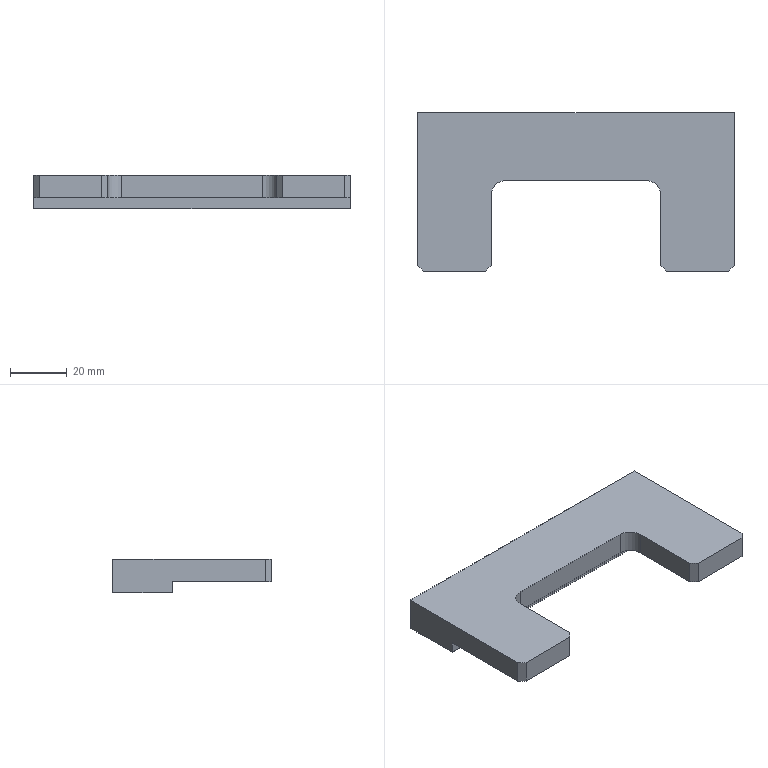Part | SolidWorks | features ICE 2, Chamfer 1, Extrusion 1, Fillet 1, HoleWzd 1 | 1 solid | 30 faces | box 112 x 56 x 12 mm | volume 43333 mm3 | plane 16 | cylinder 8 | cone 6 | commonest cylinder face diameters 5 x6 10 x2
STEP:
#1=CARTESIAN_POINT('',(6.,41.,3.5));
#2=VERTEX_POINT('',#1);
#3=CARTESIAN_POINT('',(6.,41.,8.5));
#4=VERTEX_POINT('',#3);
#5=CARTESIAN_POINT('',(6.,41.,6.));
#6=DIRECTION('',(0.,1.,0.));
#7=DIRECTION('',(0.,0.,1.));
#8=AXIS2_PLACEMENT_3D('',#5,#6,#7);
#9=CIRCLE('',#8,2.5);
#10=EDGE_CURVE('',#2,#4,#9,.T.);
#11=ORIENTED_EDGE('',*,*,#10,.F.);
#12=CARTESIAN_POINT('',(6.,56.,3.5));
#13=VERTEX_POINT('',#12);
#14=CARTESIAN_POINT('',(6.,56.,3.5));
#15=DIRECTION('',(0.,1.,0.));
#16=VECTOR('',#15,1000.);
#17=LINE('',#14,#16);
#18=EDGE_CURVE('',#2,#13,#17,.T.);
#19=ORIENTED_EDGE('',*,*,#18,.T.);
#20=CARTESIAN_POINT('',(6.,56.,8.5));
#21=VERTEX_POINT('',#20);
#22=CARTESIAN_POINT('',(6.,56.,6.));
#23=DIRECTION('',(0.,1.,0.));
#24=DIRECTION('',(0.,0.,1.));
#25=AXIS2_PLACEMENT_3D('',#22,#23,#24);
#26=CIRCLE('',#25,2.5);
#27=EDGE_CURVE('',#13,#21,#26,.T.);
#28=ORIENTED_EDGE('',*,*,#27,.T.);
#29=CARTESIAN_POINT('',(6.,56.,8.5));
#30=DIRECTION('',(0.,1.,0.));
#31=VECTOR('',#30,1000.);
#32=LINE('',#29,#31);
#33=EDGE_CURVE('',#4,#21,#32,.T.);
#34=ORIENTED_EDGE('',*,*,#33,.F.);
#35=EDGE_LOOP('',(#11,#19,#28,#34));
#36=FACE_OUTER_BOUND('',#35,.T.);
#37=CARTESIAN_POINT('',(6.,56.,6.));
#38=DIRECTION('',(0.,1.,0.));
#39=DIRECTION('',(0.,0.,1.));
#40=AXIS2_PLACEMENT_3D('',#37,#38,#39);
#41=CYLINDRICAL_SURFACE('',#40,2.5);
#42=ADVANCED_FACE('',(#36),#41,.F.);
#43=CARTESIAN_POINT('',(6.,39.498,6.));
#44=VERTEX_POINT('',#43);
#45=CARTESIAN_POINT('',(6.,41.,8.5));
#46=DIRECTION('',(0.,0.515,0.8572));
#47=VECTOR('',#46,1000.);
#48=LINE('',#45,#47);
#49=EDGE_CURVE('',#44,#4,#48,.T.);
#50=ORIENTED_EDGE('',*,*,#49,.F.);
#51=CARTESIAN_POINT('',(6.,41.,3.5));
#52=DIRECTION('',(0.,0.515,-0.8572));
#53=VECTOR('',#52,1000.);
#54=LINE('',#51,#53);
#55=EDGE_CURVE('',#44,#2,#54,.T.);
#56=ORIENTED_EDGE('',*,*,#55,.T.);
#57=ORIENTED_EDGE('',*,*,#10,.T.);
#58=EDGE_LOOP('',(#50,#56,#57));
#59=FACE_OUTER_BOUND('',#58,.T.);
#60=CARTESIAN_POINT('',(6.,41.,6.));
#61=DIRECTION('',(0.,1.,0.));
#62=DIRECTION('',(0.,0.,1.));
#63=AXIS2_PLACEMENT_3D('',#60,#61,#62);
#64=CONICAL_SURFACE('',#63,2.5,1.03);
#65=ADVANCED_FACE('',(#59),#64,.F.);
#66=CARTESIAN_POINT('',(56.,41.,3.5));
#67=VERTEX_POINT('',#66);
#68=CARTESIAN_POINT('',(56.,41.,8.5));
#69=VERTEX_POINT('',#68);
#70=CARTESIAN_POINT('',(56.,41.,6.));
#71=DIRECTION('',(0.,1.,0.));
#72=DIRECTION('',(0.,0.,1.));
#73=AXIS2_PLACEMENT_3D('',#70,#71,#72);
#74=CIRCLE('',#73,2.5);
#75=EDGE_CURVE('',#67,#69,#74,.T.);
#76=ORIENTED_EDGE('',*,*,#75,.F.);
#77=CARTESIAN_POINT('',(56.,56.,3.5));
#78=VERTEX_POINT('',#77);
#79=CARTESIAN_POINT('',(56.,56.,3.5));
#80=DIRECTION('',(0.,1.,0.));
#81=VECTOR('',#80,1000.);
#82=LINE('',#79,#81);
#83=EDGE_CURVE('',#67,#78,#82,.T.);
#84=ORIENTED_EDGE('',*,*,#83,.T.);
#85=CARTESIAN_POINT('',(56.,56.,8.5));
#86=VERTEX_POINT('',#85);
#87=CARTESIAN_POINT('',(56.,56.,6.));
#88=DIRECTION('',(0.,1.,0.));
#89=DIRECTION('',(0.,0.,1.));
#90=AXIS2_PLACEMENT_3D('',#87,#88,#89);
#91=CIRCLE('',#90,2.5);
#92=EDGE_CURVE('',#78,#86,#91,.T.);
#93=ORIENTED_EDGE('',*,*,#92,.T.);
#94=CARTESIAN_POINT('',(56.,56.,8.5));
#95=DIRECTION('',(0.,1.,0.));
#96=VECTOR('',#95,1000.);
#97=LINE('',#94,#96);
#98=EDGE_CURVE('',#69,#86,#97,.T.);
#99=ORIENTED_EDGE('',*,*,#98,.F.);
#100=EDGE_LOOP('',(#76,#84,#93,#99));
#101=FACE_OUTER_BOUND('',#100,.T.);
#102=CARTESIAN_POINT('',(56.,56.,6.));
#103=DIRECTION('',(0.,1.,0.));
#104=DIRECTION('',(0.,0.,1.));
#105=AXIS2_PLACEMENT_3D('',#102,#103,#104);
#106=CYLINDRICAL_SURFACE('',#105,2.5);
#107=ADVANCED_FACE('',(#101),#106,.F.);
#108=CARTESIAN_POINT('',(56.,39.498,6.));
#109=VERTEX_POINT('',#108);
#110=CARTESIAN_POINT('',(56.,41.,8.5));
#111=DIRECTION('',(0.,0.515,0.8572));
#112=VECTOR('',#111,1000.);
#113=LINE('',#110,#112);
#114=EDGE_CURVE('',#109,#69,#113,.T.);
#115=ORIENTED_EDGE('',*,*,#114,.F.);
#116=CARTESIAN_POINT('',(56.,41.,3.5));
#117=DIRECTION('',(0.,0.515,-0.8572));
#118=VECTOR('',#117,1000.);
#119=LINE('',#116,#118);
#120=EDGE_CURVE('',#109,#67,#119,.T.);
#121=ORIENTED_EDGE('',*,*,#120,.T.);
#122=ORIENTED_EDGE('',*,*,#75,.T.);
#123=EDGE_LOOP('',(#115,#121,#122));
#124=FACE_OUTER_BOUND('',#123,.T.);
#125=CARTESIAN_POINT('',(56.,41.,6.));
#126=DIRECTION('',(0.,1.,0.));
#127=DIRECTION('',(0.,0.,1.));
#128=AXIS2_PLACEMENT_3D('',#125,#126,#127);
#129=CONICAL_SURFACE('',#128,2.5,1.03);
#130=ADVANCED_FACE('',(#124),#129,.F.);
#131=CARTESIAN_POINT('',(106.,41.,3.5));
#132=VERTEX_POINT('',#131);
#133=CARTESIAN_POINT('',(106.,41.,8.5));
#134=VERTEX_POINT('',#133);
#135=CARTESIAN_POINT('',(106.,41.,6.));
#136=DIRECTION('',(0.,1.,0.));
#137=DIRECTION('',(0.,0.,1.));
#138=AXIS2_PLACEMENT_3D('',#135,#136,#137);
#139=CIRCLE('',#138,2.5);
#140=EDGE_CURVE('',#132,#134,#139,.T.);
#141=ORIENTED_EDGE('',*,*,#140,.F.);
#142=CARTESIAN_POINT('',(106.,56.,3.5));
#143=VERTEX_POINT('',#142);
#144=CARTESIAN_POINT('',(106.,56.,3.5));
#145=DIRECTION('',(0.,1.,0.));
#146=VECTOR('',#145,1000.);
#147=LINE('',#144,#146);
#148=EDGE_CURVE('',#132,#143,#147,.T.);
#149=ORIENTED_EDGE('',*,*,#148,.T.);
#150=CARTESIAN_POINT('',(106.,56.,8.5));
#151=VERTEX_POINT('',#150);
#152=CARTESIAN_POINT('',(106.,56.,6.));
#153=DIRECTION('',(0.,1.,0.));
#154=DIRECTION('',(0.,0.,1.));
#155=AXIS2_PLACEMENT_3D('',#152,#153,#154);
#156=CIRCLE('',#155,2.5);
#157=EDGE_CURVE('',#143,#151,#156,.T.);
#158=ORIENTED_EDGE('',*,*,#157,.T.);
#159=CARTESIAN_POINT('',(106.,56.,8.5));
#160=DIRECTION('',(0.,1.,0.));
#161=VECTOR('',#160,1000.);
#162=LINE('',#159,#161);
#163=EDGE_CURVE('',#134,#151,#162,.T.);
#164=ORIENTED_EDGE('',*,*,#163,.F.);
#165=EDGE_LOOP('',(#141,#149,#158,#164));
#166=FACE_OUTER_BOUND('',#165,.T.);
#167=CARTESIAN_POINT('',(106.,56.,6.));
#168=DIRECTION('',(0.,1.,0.));
#169=DIRECTION('',(0.,0.,1.));
#170=AXIS2_PLACEMENT_3D('',#167,#168,#169);
#171=CYLINDRICAL_SURFACE('',#170,2.5);
#172=ADVANCED_FACE('',(#166),#171,.F.);
#173=CARTESIAN_POINT('',(106.,39.498,6.));
#174=VERTEX_POINT('',#173);
#175=CARTESIAN_POINT('',(106.,41.,8.5));
#176=DIRECTION('',(0.,0.515,0.8572));
#177=VECTOR('',#176,1000.);
#178=LINE('',#175,#177);
#179=EDGE_CURVE('',#174,#134,#178,.T.);
#180=ORIENTED_EDGE('',*,*,#179,.F.);
#181=CARTESIAN_POINT('',(106.,41.,3.5));
#182=DIRECTION('',(0.,0.515,-0.8572));
#183=VECTOR('',#182,1000.);
#184=LINE('',#181,#183);
#185=EDGE_CURVE('',#174,#132,#184,.T.);
#186=ORIENTED_EDGE('',*,*,#185,.T.);
#187=ORIENTED_EDGE('',*,*,#140,.T.);
#188=EDGE_LOOP('',(#180,#186,#187));
#189=FACE_OUTER_BOUND('',#188,.T.);
#190=CARTESIAN_POINT('',(106.,41.,6.));
#191=DIRECTION('',(0.,1.,0.));
#192=DIRECTION('',(0.,0.,1.));
#193=AXIS2_PLACEMENT_3D('',#190,#191,#192);
#194=CONICAL_SURFACE('',#193,2.5,1.03);
#195=ADVANCED_FACE('',(#189),#194,.F.);
#196=CARTESIAN_POINT('',(88.,0.,12.));
#197=VERTEX_POINT('',#196);
#198=CARTESIAN_POINT('',(110.,0.,12.));
#199=VERTEX_POINT('',#198);
#200=CARTESIAN_POINT('',(0.,0.,12.));
#201=DIRECTION('',(1.,0.,0.));
#202=VECTOR('',#201,1000.);
#203=LINE('',#200,#202);
#204=EDGE_CURVE('',#197,#199,#203,.T.);
#205=ORIENTED_EDGE('',*,*,#204,.F.);
#206=CARTESIAN_POINT('',(88.,0.,4.));
#207=VERTEX_POINT('',#206);
#208=CARTESIAN_POINT('',(88.,0.,12.));
#209=DIRECTION('',(0.,0.,-1.));
#210=VECTOR('',#209,1000.);
#211=LINE('',#208,#210);
#212=EDGE_CURVE('',#197,#207,#211,.T.);
#213=ORIENTED_EDGE('',*,*,#212,.T.);
#214=CARTESIAN_POINT('',(110.,0.,4.));
#215=VERTEX_POINT('',#214);
#216=CARTESIAN_POINT('',(112.,0.,4.));
#217=DIRECTION('',(-1.,0.,0.));
#218=VECTOR('',#217,1000.);
#219=LINE('',#216,#218);
#220=EDGE_CURVE('',#215,#207,#219,.T.);
#221=ORIENTED_EDGE('',*,*,#220,.F.);
#222=CARTESIAN_POINT('',(110.,0.,12.));
#223=DIRECTION('',(0.,0.,1.));
#224=VECTOR('',#223,1000.);
#225=LINE('',#222,#224);
#226=EDGE_CURVE('',#215,#199,#225,.T.);
#227=ORIENTED_EDGE('',*,*,#226,.T.);
#228=EDGE_LOOP('',(#205,#213,#221,#227));
#229=FACE_OUTER_BOUND('',#228,.T.);
#230=CARTESIAN_POINT('',(0.,0.,12.));
#231=DIRECTION('',(0.,1.,0.));
#232=DIRECTION('',(0.,0.,1.));
#233=AXIS2_PLACEMENT_3D('',#230,#231,#232);
#234=PLANE('',#233);
#235=ADVANCED_FACE('',(#229),#234,.F.);
#236=CARTESIAN_POINT('',(0.,2.,4.));
#237=VERTEX_POINT('',#236);
#238=CARTESIAN_POINT('',(0.,35.,4.));
#239=VERTEX_POINT('',#238);
#240=CARTESIAN_POINT('',(0.,0.,4.));
#241=DIRECTION('',(0.,1.,0.));
#242=VECTOR('',#241,1000.);
#243=LINE('',#240,#242);
#244=EDGE_CURVE('',#237,#239,#243,.T.);
#245=ORIENTED_EDGE('',*,*,#244,.F.);
#246=CARTESIAN_POINT('',(0.,2.,12.));
#247=VERTEX_POINT('',#246);
#248=CARTESIAN_POINT('',(0.,2.,12.));
#249=DIRECTION('',(0.,0.,1.));
#250=VECTOR('',#249,1000.);
#251=LINE('',#248,#250);
#252=EDGE_CURVE('',#237,#247,#251,.T.);
#253=ORIENTED_EDGE('',*,*,#252,.T.);
#254=CARTESIAN_POINT('',(0.,56.,12.));
#255=VERTEX_POINT('',#254);
#256=CARTESIAN_POINT('',(0.,0.,12.));
#257=DIRECTION('',(0.,-1.,0.));
#258=VECTOR('',#257,1000.);
#259=LINE('',#256,#258);
#260=EDGE_CURVE('',#255,#247,#259,.T.);
#261=ORIENTED_EDGE('',*,*,#260,.F.);
#262=CARTESIAN_POINT('',(0.,56.,0.));
#263=VERTEX_POINT('',#262);
#264=CARTESIAN_POINT('',(0.,56.,12.));
#265=DIRECTION('',(0.,0.,-1.));
#266=VECTOR('',#265,1000.);
#267=LINE('',#264,#266);
#268=EDGE_CURVE('',#255,#263,#267,.T.);
#269=ORIENTED_EDGE('',*,*,#268,.T.);
#270=CARTESIAN_POINT('',(0.,35.,0.));
#271=VERTEX_POINT('',#270);
#272=CARTESIAN_POINT('',(0.,0.,0.));
#273=DIRECTION('',(0.,-1.,0.));
#274=VECTOR('',#273,1000.);
#275=LINE('',#272,#274);
#276=EDGE_CURVE('',#263,#271,#275,.T.);
#277=ORIENTED_EDGE('',*,*,#276,.T.);
#278=CARTESIAN_POINT('',(0.,35.,4.));
#279=DIRECTION('',(0.,0.,-1.));
#280=VECTOR('',#279,1000.);
#281=LINE('',#278,#280);
#282=EDGE_CURVE('',#239,#271,#281,.T.);
#283=ORIENTED_EDGE('',*,*,#282,.F.);
#284=EDGE_LOOP('',(#245,#253,#261,#269,#277,#283));
#285=FACE_OUTER_BOUND('',#284,.T.);
#286=CARTESIAN_POINT('',(0.,0.,12.));
#287=DIRECTION('',(1.,0.,0.));
#288=DIRECTION('',(0.,0.,-1.));
#289=AXIS2_PLACEMENT_3D('',#286,#287,#288);
#290=PLANE('',#289);
#291=ADVANCED_FACE('',(#285),#290,.F.);
#292=CARTESIAN_POINT('',(2.,0.,12.));
#293=VERTEX_POINT('',#292);
#294=CARTESIAN_POINT('',(24.,0.,12.));
#295=VERTEX_POINT('',#294);
#296=CARTESIAN_POINT('',(0.,0.,12.));
#297=DIRECTION('',(1.,0.,0.));
#298=VECTOR('',#297,1000.);
#299=LINE('',#296,#298);
#300=EDGE_CURVE('',#293,#295,#299,.T.);
#301=ORIENTED_EDGE('',*,*,#300,.F.);
#302=CARTESIAN_POINT('',(2.,0.,4.));
#303=VERTEX_POINT('',#302);
#304=CARTESIAN_POINT('',(2.,0.,12.));
#305=DIRECTION('',(0.,0.,-1.));
#306=VECTOR('',#305,1000.);
#307=LINE('',#304,#306);
#308=EDGE_CURVE('',#293,#303,#307,.T.);
#309=ORIENTED_EDGE('',*,*,#308,.T.);
#310=CARTESIAN_POINT('',(24.,0.,4.));
#311=VERTEX_POINT('',#310);
#312=CARTESIAN_POINT('',(112.,0.,4.));
#313=DIRECTION('',(-1.,0.,0.));
#314=VECTOR('',#313,1000.);
#315=LINE('',#312,#314);
#316=EDGE_CURVE('',#311,#303,#315,.T.);
#317=ORIENTED_EDGE('',*,*,#316,.F.);
#318=CARTESIAN_POINT('',(24.,0.,12.));
#319=DIRECTION('',(0.,0.,1.));
#320=VECTOR('',#319,1000.);
#321=LINE('',#318,#320);
#322=EDGE_CURVE('',#311,#295,#321,.T.);
#323=ORIENTED_EDGE('',*,*,#322,.T.);
#324=EDGE_LOOP('',(#301,#309,#317,#323));
#325=FACE_OUTER_BOUND('',#324,.T.);
#326=CARTESIAN_POINT('',(0.,0.,12.));
#327=DIRECTION('',(0.,1.,0.));
#328=DIRECTION('',(0.,0.,1.));
#329=AXIS2_PLACEMENT_3D('',#326,#327,#328);
#330=PLANE('',#329);
#331=ADVANCED_FACE('',(#325),#330,.F.);
#332=CARTESIAN_POINT('',(112.,2.,12.));
#333=VERTEX_POINT('',#332);
#334=CARTESIAN_POINT('',(112.,56.,12.));
#335=VERTEX_POINT('',#334);
#336=CARTESIAN_POINT('',(112.,0.,12.));
#337=DIRECTION('',(0.,1.,0.));
#338=VECTOR('',#337,1000.);
#339=LINE('',#336,#338);
#340=EDGE_CURVE('',#333,#335,#339,.T.);
#341=ORIENTED_EDGE('',*,*,#340,.F.);
#342=CARTESIAN_POINT('',(112.,2.,4.));
#343=VERTEX_POINT('',#342);
#344=CARTESIAN_POINT('',(112.,2.,12.));
#345=DIRECTION('',(0.,0.,-1.));
#346=VECTOR('',#345,1000.);
#347=LINE('',#344,#346);
#348=EDGE_CURVE('',#333,#343,#347,.T.);
#349=ORIENTED_EDGE('',*,*,#348,.T.);
#350=CARTESIAN_POINT('',(112.,35.,4.));
#351=VERTEX_POINT('',#350);
#352=CARTESIAN_POINT('',(112.,0.,4.));
#353=DIRECTION('',(0.,-1.,0.));
#354=VECTOR('',#353,1000.);
#355=LINE('',#352,#354);
#356=EDGE_CURVE('',#351,#343,#355,.T.);
#357=ORIENTED_EDGE('',*,*,#356,.F.);
#358=CARTESIAN_POINT('',(112.,35.,0.));
#359=VERTEX_POINT('',#358);
#360=CARTESIAN_POINT('',(112.,35.,4.));
#361=DIRECTION('',(0.,0.,-1.));
#362=VECTOR('',#361,1000.);
#363=LINE('',#360,#362);
#364=EDGE_CURVE('',#351,#359,#363,.T.);
#365=ORIENTED_EDGE('',*,*,#364,.T.);
#366=CARTESIAN_POINT('',(112.,56.,0.));
#367=VERTEX_POINT('',#366);
#368=CARTESIAN_POINT('',(112.,0.,0.));
#369=DIRECTION('',(0.,1.,0.));
#370=VECTOR('',#369,1000.);
#371=LINE('',#368,#370);
#372=EDGE_CURVE('',#359,#367,#371,.T.);
#373=ORIENTED_EDGE('',*,*,#372,.T.);
#374=CARTESIAN_POINT('',(112.,56.,12.));
#375=DIRECTION('',(0.,0.,-1.));
#376=VECTOR('',#375,1000.);
#377=LINE('',#374,#376);
#378=EDGE_CURVE('',#335,#367,#377,.T.);
#379=ORIENTED_EDGE('',*,*,#378,.F.);
#380=EDGE_LOOP('',(#341,#349,#357,#365,#373,#379));
#381=FACE_OUTER_BOUND('',#380,.T.);
#382=CARTESIAN_POINT('',(112.,0.,12.));
#383=DIRECTION('',(-1.,0.,0.));
#384=DIRECTION('',(0.,0.,1.));
#385=AXIS2_PLACEMENT_3D('',#382,#383,#384);
#386=PLANE('',#385);
#387=ADVANCED_FACE('',(#381),#386,.F.);
#388=CARTESIAN_POINT('',(6.,56.,6.));
#389=DIRECTION('',(0.,1.,0.));
#390=DIRECTION('',(0.,0.,1.));
#391=AXIS2_PLACEMENT_3D('',#388,#389,#390);
#392=CIRCLE('',#391,2.5);
#393=EDGE_CURVE('',#21,#13,#392,.T.);
#394=ORIENTED_EDGE('',*,*,#393,.F.);
#395=ORIENTED_EDGE('',*,*,#27,.F.);
#396=EDGE_LOOP('',(#394,#395));
#397=FACE_BOUND('',#396,.T.);
#398=CARTESIAN_POINT('',(56.,56.,6.));
#399=DIRECTION('',(0.,1.,0.));
#400=DIRECTION('',(0.,0.,1.));
#401=AXIS2_PLACEMENT_3D('',#398,#399,#400);
#402=CIRCLE('',#401,2.5);
#403=EDGE_CURVE('',#86,#78,#402,.T.);
#404=ORIENTED_EDGE('',*,*,#403,.F.);
#405=ORIENTED_EDGE('',*,*,#92,.F.);
#406=EDGE_LOOP('',(#404,#405));
#407=FACE_BOUND('',#406,.T.);
#408=CARTESIAN_POINT('',(106.,56.,6.));
#409=DIRECTION('',(0.,1.,0.));
#410=DIRECTION('',(0.,0.,1.));
#411=AXIS2_PLACEMENT_3D('',#408,#409,#410);
#412=CIRCLE('',#411,2.5);
#413=EDGE_CURVE('',#151,#143,#412,.T.);
#414=ORIENTED_EDGE('',*,*,#413,.F.);
#415=ORIENTED_EDGE('',*,*,#157,.F.);
#416=EDGE_LOOP('',(#414,#415));
#417=FACE_BOUND('',#416,.T.);
#418=CARTESIAN_POINT('',(0.,56.,0.));
#419=DIRECTION('',(-1.,0.,0.));
#420=VECTOR('',#419,1000.);
#421=LINE('',#418,#420);
#422=EDGE_CURVE('',#367,#263,#421,.T.);
#423=ORIENTED_EDGE('',*,*,#422,.T.);
#424=ORIENTED_EDGE('',*,*,#268,.F.);
#425=CARTESIAN_POINT('',(0.,56.,12.));
#426=DIRECTION('',(-1.,0.,0.));
#427=VECTOR('',#426,1000.);
#428=LINE('',#425,#427);
#429=EDGE_CURVE('',#335,#255,#428,.T.);
#430=ORIENTED_EDGE('',*,*,#429,.F.);
#431=ORIENTED_EDGE('',*,*,#378,.T.);
#432=EDGE_LOOP('',(#423,#424,#430,#431));
#433=FACE_OUTER_BOUND('',#432,.T.);
#434=CARTESIAN_POINT('',(0.,56.,12.));
#435=DIRECTION('',(0.,-1.,0.));
#436=DIRECTION('',(0.,0.,-1.));
#437=AXIS2_PLACEMENT_3D('',#434,#435,#436);
#438=PLANE('',#437);
#439=ADVANCED_FACE('',(#397,#407,#417,#433),#438,.F.);
#440=ORIENTED_EDGE('',*,*,#260,.T.);
#441=CARTESIAN_POINT('',(2.,0.,12.));
#442=DIRECTION('',(0.7071,-0.7071,0.));
#443=VECTOR('',#442,1000.);
#444=LINE('',#441,#443);
#445=EDGE_CURVE('',#247,#293,#444,.T.);
#446=ORIENTED_EDGE('',*,*,#445,.T.);
#447=ORIENTED_EDGE('',*,*,#300,.T.);
#448=CARTESIAN_POINT('',(26.,2.,12.));
#449=VERTEX_POINT('',#448);
#450=CARTESIAN_POINT('',(26.,2.,12.));
#451=DIRECTION('',(0.7071,0.7071,0.));
#452=VECTOR('',#451,1000.);
#453=LINE('',#450,#452);
#454=EDGE_CURVE('',#295,#449,#453,.T.);
#455=ORIENTED_EDGE('',*,*,#454,.T.);
#456=CARTESIAN_POINT('',(26.,27.,12.));
#457=VERTEX_POINT('',#456);
#458=CARTESIAN_POINT('',(26.,0.,12.));
#459=DIRECTION('',(0.,1.,0.));
#460=VECTOR('',#459,1000.);
#461=LINE('',#458,#460);
#462=EDGE_CURVE('',#449,#457,#461,.T.);
#463=ORIENTED_EDGE('',*,*,#462,.T.);
#464=CARTESIAN_POINT('',(31.,32.,12.));
#465=VERTEX_POINT('',#464);
#466=CARTESIAN_POINT('',(31.,27.,12.));
#467=DIRECTION('',(0.,0.,-1.));
#468=DIRECTION('',(-1.,0.,0.));
#469=AXIS2_PLACEMENT_3D('',#466,#467,#468);
#470=CIRCLE('',#469,5.);
#471=EDGE_CURVE('',#457,#465,#470,.T.);
#472=ORIENTED_EDGE('',*,*,#471,.T.);
#473=CARTESIAN_POINT('',(81.,32.,12.));
#474=VERTEX_POINT('',#473);
#475=CARTESIAN_POINT('',(86.,32.,12.));
#476=DIRECTION('',(1.,0.,0.));
#477=VECTOR('',#476,1000.);
#478=LINE('',#475,#477);
#479=EDGE_CURVE('',#465,#474,#478,.T.);
#480=ORIENTED_EDGE('',*,*,#479,.T.);
#481=CARTESIAN_POINT('',(86.,27.,12.));
#482=VERTEX_POINT('',#481);
#483=CARTESIAN_POINT('',(81.,27.,12.));
#484=DIRECTION('',(0.,0.,-1.));
#485=DIRECTION('',(-1.,0.,0.));
#486=AXIS2_PLACEMENT_3D('',#483,#484,#485);
#487=CIRCLE('',#486,5.);
#488=EDGE_CURVE('',#474,#482,#487,.T.);
#489=ORIENTED_EDGE('',*,*,#488,.T.);
#490=CARTESIAN_POINT('',(86.,2.,12.));
#491=VERTEX_POINT('',#490);
#492=CARTESIAN_POINT('',(86.,0.,12.));
#493=DIRECTION('',(0.,-1.,0.));
#494=VECTOR('',#493,1000.);
#495=LINE('',#492,#494);
#496=EDGE_CURVE('',#482,#491,#495,.T.);
#497=ORIENTED_EDGE('',*,*,#496,.T.);
#498=CARTESIAN_POINT('',(88.,0.,12.));
#499=DIRECTION('',(0.7071,-0.7071,0.));
#500=VECTOR('',#499,1000.);
#501=LINE('',#498,#500);
#502=EDGE_CURVE('',#491,#197,#501,.T.);
#503=ORIENTED_EDGE('',*,*,#502,.T.);
#504=ORIENTED_EDGE('',*,*,#204,.T.);
#505=CARTESIAN_POINT('',(112.,2.,12.));
#506=DIRECTION('',(0.7071,0.7071,0.));
#507=VECTOR('',#506,1000.);
#508=LINE('',#505,#507);
#509=EDGE_CURVE('',#199,#333,#508,.T.);
#510=ORIENTED_EDGE('',*,*,#509,.T.);
#511=ORIENTED_EDGE('',*,*,#340,.T.);
#512=ORIENTED_EDGE('',*,*,#429,.T.);
#513=EDGE_LOOP('',(#440,#446,#447,#455,#463,#472,#480,#489,#497,#503,#504,#510,#511,#512));
#514=FACE_OUTER_BOUND('',#513,.T.);
#515=CARTESIAN_POINT('',(0.,0.,12.));
#516=DIRECTION('',(0.,0.,-1.));
#517=DIRECTION('',(-1.,0.,0.));
#518=AXIS2_PLACEMENT_3D('',#515,#516,#517);
#519=PLANE('',#518);
#520=ADVANCED_FACE('',(#514),#519,.F.);
#521=CARTESIAN_POINT('',(112.,35.,0.));
#522=DIRECTION('',(1.,0.,0.));
#523=VECTOR('',#522,1000.);
#524=LINE('',#521,#523);
#525=EDGE_CURVE('',#271,#359,#524,.T.);
#526=ORIENTED_EDGE('',*,*,#525,.F.);
#527=ORIENTED_EDGE('',*,*,#276,.F.);
#528=ORIENTED_EDGE('',*,*,#422,.F.);
#529=ORIENTED_EDGE('',*,*,#372,.F.);
#530=EDGE_LOOP('',(#526,#527,#528,#529));
#531=FACE_OUTER_BOUND('',#530,.T.);
#532=CARTESIAN_POINT('',(0.,0.,0.));
#533=DIRECTION('',(0.,0.,-1.));
#534=DIRECTION('',(-1.,0.,0.));
#535=AXIS2_PLACEMENT_3D('',#532,#533,#534);
#536=PLANE('',#535);
#537=ADVANCED_FACE('',(#531),#536,.T.);
#538=ORIENTED_EDGE('',*,*,#525,.T.);
#539=ORIENTED_EDGE('',*,*,#364,.F.);
#540=CARTESIAN_POINT('',(112.,35.,4.));
#541=DIRECTION('',(1.,0.,0.));
#542=VECTOR('',#541,1000.);
#543=LINE('',#540,#542);
#544=EDGE_CURVE('',#239,#351,#543,.T.);
#545=ORIENTED_EDGE('',*,*,#544,.F.);
#546=ORIENTED_EDGE('',*,*,#282,.T.);
#547=EDGE_LOOP('',(#538,#539,#545,#546));
#548=FACE_OUTER_BOUND('',#547,.T.);
#549=CARTESIAN_POINT('',(112.,35.,4.));
#550=DIRECTION('',(0.,1.,0.));
#551=DIRECTION('',(0.,0.,1.));
#552=AXIS2_PLACEMENT_3D('',#549,#550,#551);
#553=PLANE('',#552);
#554=ADVANCED_FACE('',(#548),#553,.F.);
#555=ORIENTED_EDGE('',*,*,#316,.T.);
#556=CARTESIAN_POINT('',(2.,0.,4.));
#557=DIRECTION('',(-0.7071,0.7071,0.));
#558=VECTOR('',#557,1000.);
#559=LINE('',#556,#558);
#560=EDGE_CURVE('',#303,#237,#559,.T.);
#561=ORIENTED_EDGE('',*,*,#560,.T.);
#562=ORIENTED_EDGE('',*,*,#244,.T.);
#563=ORIENTED_EDGE('',*,*,#544,.T.);
#564=ORIENTED_EDGE('',*,*,#356,.T.);
#565=CARTESIAN_POINT('',(112.,2.,4.));
#566=DIRECTION('',(-0.7071,-0.7071,0.));
#567=VECTOR('',#566,1000.);
#568=LINE('',#565,#567);
#569=EDGE_CURVE('',#343,#215,#568,.T.);
#570=ORIENTED_EDGE('',*,*,#569,.T.);
#571=ORIENTED_EDGE('',*,*,#220,.T.);
#572=CARTESIAN_POINT('',(86.,2.,4.));
#573=VERTEX_POINT('',#572);
#574=CARTESIAN_POINT('',(88.,0.,4.));
#575=DIRECTION('',(-0.7071,0.7071,0.));
#576=VECTOR('',#575,1000.);
#577=LINE('',#574,#576);
#578=EDGE_CURVE('',#207,#573,#577,.T.);
#579=ORIENTED_EDGE('',*,*,#578,.T.);
#580=CARTESIAN_POINT('',(86.,27.,4.));
#581=VERTEX_POINT('',#580);
#582=CARTESIAN_POINT('',(86.,0.,4.));
#583=DIRECTION('',(0.,-1.,0.));
#584=VECTOR('',#583,1000.);
#585=LINE('',#582,#584);
#586=EDGE_CURVE('',#581,#573,#585,.T.);
#587=ORIENTED_EDGE('',*,*,#586,.F.);
#588=CARTESIAN_POINT('',(81.,32.,4.));
#589=VERTEX_POINT('',#588);
#590=CARTESIAN_POINT('',(81.,27.,4.));
#591=DIRECTION('',(0.,0.,1.));
#592=DIRECTION('',(1.,0.,0.));
#593=AXIS2_PLACEMENT_3D('',#590,#591,#592);
#594=CIRCLE('',#593,5.);
#595=EDGE_CURVE('',#581,#589,#594,.T.);
#596=ORIENTED_EDGE('',*,*,#595,.T.);
#597=CARTESIAN_POINT('',(31.,32.,4.));
#598=VERTEX_POINT('',#597);
#599=CARTESIAN_POINT('',(86.,32.,4.));
#600=DIRECTION('',(1.,0.,0.));
#601=VECTOR('',#600,1000.);
#602=LINE('',#599,#601);
#603=EDGE_CURVE('',#598,#589,#602,.T.);
#604=ORIENTED_EDGE('',*,*,#603,.F.);
#605=CARTESIAN_POINT('',(26.,27.,4.));
#606=VERTEX_POINT('',#605);
#607=CARTESIAN_POINT('',(31.,27.,4.));
#608=DIRECTION('',(0.,0.,1.));
#609=DIRECTION('',(1.,0.,0.));
#610=AXIS2_PLACEMENT_3D('',#607,#608,#609);
#611=CIRCLE('',#610,5.);
#612=EDGE_CURVE('',#598,#606,#611,.T.);
#613=ORIENTED_EDGE('',*,*,#612,.T.);
#614=CARTESIAN_POINT('',(26.,2.,4.));
#615=VERTEX_POINT('',#614);
#616=CARTESIAN_POINT('',(26.,0.,4.));
#617=DIRECTION('',(0.,1.,0.));
#618=VECTOR('',#617,1000.);
#619=LINE('',#616,#618);
#620=EDGE_CURVE('',#615,#606,#619,.T.);
#621=ORIENTED_EDGE('',*,*,#620,.F.);
#622=CARTESIAN_POINT('',(26.,2.,4.));
#623=DIRECTION('',(-0.7071,-0.7071,0.));
#624=VECTOR('',#623,1000.);
#625=LINE('',#622,#624);
#626=EDGE_CURVE('',#615,#311,#625,.T.);
#627=ORIENTED_EDGE('',*,*,#626,.T.);
#628=EDGE_LOOP('',(#555,#561,#562,#563,#564,#570,#571,#579,#587,#596,#604,#613,#621,#627));
#629=FACE_OUTER_BOUND('',#628,.T.);
#630=CARTESIAN_POINT('',(0.,0.,4.));
#631=DIRECTION('',(0.,0.,1.));
#632=DIRECTION('',(1.,0.,0.));
#633=AXIS2_PLACEMENT_3D('',#630,#631,#632);
#634=PLANE('',#633);
#635=ADVANCED_FACE('',(#629),#634,.F.);
#636=ORIENTED_EDGE('',*,*,#185,.F.);
#637=ORIENTED_EDGE('',*,*,#179,.T.);
#638=CARTESIAN_POINT('',(106.,41.,6.));
#639=DIRECTION('',(0.,1.,0.));
#640=DIRECTION('',(0.,0.,1.));
#641=AXIS2_PLACEMENT_3D('',#638,#639,#640);
#642=CIRCLE('',#641,2.5);
#643=EDGE_CURVE('',#134,#132,#642,.T.);
#644=ORIENTED_EDGE('',*,*,#643,.T.);
#645=EDGE_LOOP('',(#636,#637,#644));
#646=FACE_OUTER_BOUND('',#645,.T.);
#647=CARTESIAN_POINT('',(106.,41.,6.));
#648=DIRECTION('',(0.,1.,0.));
#649=DIRECTION('',(0.,0.,1.));
#650=AXIS2_PLACEMENT_3D('',#647,#648,#649);
#651=CONICAL_SURFACE('',#650,2.5,1.03);
#652=ADVANCED_FACE('',(#646),#651,.F.);
#653=ORIENTED_EDGE('',*,*,#148,.F.);
#654=ORIENTED_EDGE('',*,*,#643,.F.);
#655=ORIENTED_EDGE('',*,*,#163,.T.);
#656=ORIENTED_EDGE('',*,*,#413,.T.);
#657=EDGE_LOOP('',(#653,#654,#655,#656));
#658=FACE_OUTER_BOUND('',#657,.T.);
#659=CARTESIAN_POINT('',(106.,56.,6.));
#660=DIRECTION('',(0.,1.,0.));
#661=DIRECTION('',(0.,0.,1.));
#662=AXIS2_PLACEMENT_3D('',#659,#660,#661);
#663=CYLINDRICAL_SURFACE('',#662,2.5);
#664=ADVANCED_FACE('',(#658),#663,.F.);
#665=ORIENTED_EDGE('',*,*,#120,.F.);
#666=ORIENTED_EDGE('',*,*,#114,.T.);
#667=CARTESIAN_POINT('',(56.,41.,6.));
#668=DIRECTION('',(0.,1.,0.));
#669=DIRECTION('',(0.,0.,1.));
#670=AXIS2_PLACEMENT_3D('',#667,#668,#669);
#671=CIRCLE('',#670,2.5);
#672=EDGE_CURVE('',#69,#67,#671,.T.);
#673=ORIENTED_EDGE('',*,*,#672,.T.);
#674=EDGE_LOOP('',(#665,#666,#673));
#675=FACE_OUTER_BOUND('',#674,.T.);
#676=CARTESIAN_POINT('',(56.,41.,6.));
#677=DIRECTION('',(0.,1.,0.));
#678=DIRECTION('',(0.,0.,1.));
#679=AXIS2_PLACEMENT_3D('',#676,#677,#678);
#680=CONICAL_SURFACE('',#679,2.5,1.03);
#681=ADVANCED_FACE('',(#675),#680,.F.);
#682=ORIENTED_EDGE('',*,*,#83,.F.);
#683=ORIENTED_EDGE('',*,*,#672,.F.);
#684=ORIENTED_EDGE('',*,*,#98,.T.);
#685=ORIENTED_EDGE('',*,*,#403,.T.);
#686=EDGE_LOOP('',(#682,#683,#684,#685));
#687=FACE_OUTER_BOUND('',#686,.T.);
#688=CARTESIAN_POINT('',(56.,56.,6.));
#689=DIRECTION('',(0.,1.,0.));
#690=DIRECTION('',(0.,0.,1.));
#691=AXIS2_PLACEMENT_3D('',#688,#689,#690);
#692=CYLINDRICAL_SURFACE('',#691,2.5);
#693=ADVANCED_FACE('',(#687),#692,.F.);
#694=ORIENTED_EDGE('',*,*,#55,.F.);
#695=ORIENTED_EDGE('',*,*,#49,.T.);
#696=CARTESIAN_POINT('',(6.,41.,6.));
#697=DIRECTION('',(0.,1.,0.));
#698=DIRECTION('',(0.,0.,1.));
#699=AXIS2_PLACEMENT_3D('',#696,#697,#698);
#700=CIRCLE('',#699,2.5);
#701=EDGE_CURVE('',#4,#2,#700,.T.);
#702=ORIENTED_EDGE('',*,*,#701,.T.);
#703=EDGE_LOOP('',(#694,#695,#702));
#704=FACE_OUTER_BOUND('',#703,.T.);
#705=CARTESIAN_POINT('',(6.,41.,6.));
#706=DIRECTION('',(0.,1.,0.));
#707=DIRECTION('',(0.,0.,1.));
#708=AXIS2_PLACEMENT_3D('',#705,#706,#707);
#709=CONICAL_SURFACE('',#708,2.5,1.03);
#710=ADVANCED_FACE('',(#704),#709,.F.);
#711=ORIENTED_EDGE('',*,*,#18,.F.);
#712=ORIENTED_EDGE('',*,*,#701,.F.);
#713=ORIENTED_EDGE('',*,*,#33,.T.);
#714=ORIENTED_EDGE('',*,*,#393,.T.);
#715=EDGE_LOOP('',(#711,#712,#713,#714));
#716=FACE_OUTER_BOUND('',#715,.T.);
#717=CARTESIAN_POINT('',(6.,56.,6.));
#718=DIRECTION('',(0.,1.,0.));
#719=DIRECTION('',(0.,0.,1.));
#720=AXIS2_PLACEMENT_3D('',#717,#718,#719);
#721=CYLINDRICAL_SURFACE('',#720,2.5);
#722=ADVANCED_FACE('',(#716),#721,.F.);
#723=ORIENTED_EDGE('',*,*,#586,.T.);
#724=CARTESIAN_POINT('',(86.,2.,12.));
#725=DIRECTION('',(0.,0.,1.));
#726=VECTOR('',#725,1000.);
#727=LINE('',#724,#726);
#728=EDGE_CURVE('',#573,#491,#727,.T.);
#729=ORIENTED_EDGE('',*,*,#728,.T.);
#730=ORIENTED_EDGE('',*,*,#496,.F.);
#731=CARTESIAN_POINT('',(86.,27.,4.));
#732=DIRECTION('',(0.,0.,-1.));
#733=VECTOR('',#732,1000.);
#734=LINE('',#731,#733);
#735=EDGE_CURVE('',#482,#581,#734,.T.);
#736=ORIENTED_EDGE('',*,*,#735,.T.);
#737=EDGE_LOOP('',(#723,#729,#730,#736));
#738=FACE_OUTER_BOUND('',#737,.T.);
#739=CARTESIAN_POINT('',(86.,0.,12.));
#740=DIRECTION('',(1.,0.,0.));
#741=DIRECTION('',(0.,0.,-1.));
#742=AXIS2_PLACEMENT_3D('',#739,#740,#741);
#743=PLANE('',#742);
#744=ADVANCED_FACE('',(#738),#743,.F.);
#745=ORIENTED_EDGE('',*,*,#479,.F.);
#746=CARTESIAN_POINT('',(31.,32.,4.));
#747=DIRECTION('',(0.,0.,-1.));
#748=VECTOR('',#747,1000.);
#749=LINE('',#746,#748);
#750=EDGE_CURVE('',#465,#598,#749,.T.);
#751=ORIENTED_EDGE('',*,*,#750,.T.);
#752=ORIENTED_EDGE('',*,*,#603,.T.);
#753=CARTESIAN_POINT('',(81.,32.,12.));
#754=DIRECTION('',(0.,0.,1.));
#755=VECTOR('',#754,1000.);
#756=LINE('',#753,#755);
#757=EDGE_CURVE('',#589,#474,#756,.T.);
#758=ORIENTED_EDGE('',*,*,#757,.T.);
#759=EDGE_LOOP('',(#745,#751,#752,#758));
#760=FACE_OUTER_BOUND('',#759,.T.);
#761=CARTESIAN_POINT('',(86.,32.,12.));
#762=DIRECTION('',(0.,1.,0.));
#763=DIRECTION('',(-1.,0.,0.));
#764=AXIS2_PLACEMENT_3D('',#761,#762,#763);
#765=PLANE('',#764);
#766=ADVANCED_FACE('',(#760),#765,.F.);
#767=ORIENTED_EDGE('',*,*,#462,.F.);
#768=CARTESIAN_POINT('',(26.,2.,12.));
#769=DIRECTION('',(0.,0.,-1.));
#770=VECTOR('',#769,1000.);
#771=LINE('',#768,#770);
#772=EDGE_CURVE('',#449,#615,#771,.T.);
#773=ORIENTED_EDGE('',*,*,#772,.T.);
#774=ORIENTED_EDGE('',*,*,#620,.T.);
#775=CARTESIAN_POINT('',(26.,27.,12.));
#776=DIRECTION('',(0.,0.,1.));
#777=VECTOR('',#776,1000.);
#778=LINE('',#775,#777);
#779=EDGE_CURVE('',#606,#457,#778,.T.);
#780=ORIENTED_EDGE('',*,*,#779,.T.);
#781=EDGE_LOOP('',(#767,#773,#774,#780));
#782=FACE_OUTER_BOUND('',#781,.T.);
#783=CARTESIAN_POINT('',(26.,0.,12.));
#784=DIRECTION('',(-1.,0.,0.));
#785=DIRECTION('',(0.,-1.,0.));
#786=AXIS2_PLACEMENT_3D('',#783,#784,#785);
#787=PLANE('',#786);
#788=ADVANCED_FACE('',(#782),#787,.F.);
#789=ORIENTED_EDGE('',*,*,#471,.F.);
#790=ORIENTED_EDGE('',*,*,#779,.F.);
#791=ORIENTED_EDGE('',*,*,#612,.F.);
#792=ORIENTED_EDGE('',*,*,#750,.F.);
#793=EDGE_LOOP('',(#789,#790,#791,#792));
#794=FACE_OUTER_BOUND('',#793,.T.);
#795=CARTESIAN_POINT('',(31.,27.,12.));
#796=DIRECTION('',(0.,0.,1.));
#797=DIRECTION('',(1.,0.,0.));
#798=AXIS2_PLACEMENT_3D('',#795,#796,#797);
#799=CYLINDRICAL_SURFACE('',#798,5.);
#800=ADVANCED_FACE('',(#794),#799,.F.);
#801=ORIENTED_EDGE('',*,*,#488,.F.);
#802=ORIENTED_EDGE('',*,*,#757,.F.);
#803=ORIENTED_EDGE('',*,*,#595,.F.);
#804=ORIENTED_EDGE('',*,*,#735,.F.);
#805=EDGE_LOOP('',(#801,#802,#803,#804));
#806=FACE_OUTER_BOUND('',#805,.T.);
#807=CARTESIAN_POINT('',(81.,27.,12.));
#808=DIRECTION('',(0.,0.,1.));
#809=DIRECTION('',(1.,0.,0.));
#810=AXIS2_PLACEMENT_3D('',#807,#808,#809);
#811=CYLINDRICAL_SURFACE('',#810,5.);
#812=ADVANCED_FACE('',(#806),#811,.F.);
#813=ORIENTED_EDGE('',*,*,#445,.F.);
#814=ORIENTED_EDGE('',*,*,#252,.F.);
#815=ORIENTED_EDGE('',*,*,#560,.F.);
#816=ORIENTED_EDGE('',*,*,#308,.F.);
#817=EDGE_LOOP('',(#813,#814,#815,#816));
#818=FACE_OUTER_BOUND('',#817,.T.);
#819=CARTESIAN_POINT('',(2.,0.,12.));
#820=DIRECTION('',(0.7071,0.7071,0.));
#821=DIRECTION('',(0.,0.,-1.));
#822=AXIS2_PLACEMENT_3D('',#819,#820,#821);
#823=PLANE('',#822);
#824=ADVANCED_FACE('',(#818),#823,.F.);
#825=ORIENTED_EDGE('',*,*,#454,.F.);
#826=ORIENTED_EDGE('',*,*,#322,.F.);
#827=ORIENTED_EDGE('',*,*,#626,.F.);
#828=ORIENTED_EDGE('',*,*,#772,.F.);
#829=EDGE_LOOP('',(#825,#826,#827,#828));
#830=FACE_OUTER_BOUND('',#829,.T.);
#831=CARTESIAN_POINT('',(26.,2.,12.));
#832=DIRECTION('',(-0.7071,0.7071,0.));
#833=DIRECTION('',(0.,0.,-1.));
#834=AXIS2_PLACEMENT_3D('',#831,#832,#833);
#835=PLANE('',#834);
#836=ADVANCED_FACE('',(#830),#835,.F.);
#837=ORIENTED_EDGE('',*,*,#502,.F.);
#838=ORIENTED_EDGE('',*,*,#728,.F.);
#839=ORIENTED_EDGE('',*,*,#578,.F.);
#840=ORIENTED_EDGE('',*,*,#212,.F.);
#841=EDGE_LOOP('',(#837,#838,#839,#840));
#842=FACE_OUTER_BOUND('',#841,.T.);
#843=CARTESIAN_POINT('',(88.,0.,12.));
#844=DIRECTION('',(0.7071,0.7071,0.));
#845=DIRECTION('',(0.,0.,-1.));
#846=AXIS2_PLACEMENT_3D('',#843,#844,#845);
#847=PLANE('',#846);
#848=ADVANCED_FACE('',(#842),#847,.F.);
#849=ORIENTED_EDGE('',*,*,#509,.F.);
#850=ORIENTED_EDGE('',*,*,#226,.F.);
#851=ORIENTED_EDGE('',*,*,#569,.F.);
#852=ORIENTED_EDGE('',*,*,#348,.F.);
#853=EDGE_LOOP('',(#849,#850,#851,#852));
#854=FACE_OUTER_BOUND('',#853,.T.);
#855=CARTESIAN_POINT('',(112.,2.,12.));
#856=DIRECTION('',(-0.7071,0.7071,0.));
#857=DIRECTION('',(0.,0.,-1.));
#858=AXIS2_PLACEMENT_3D('',#855,#856,#857);
#859=PLANE('',#858);
#860=ADVANCED_FACE('',(#854),#859,.F.);
#861=CLOSED_SHELL('',(#42,#65,#107,#130,#172,#195,#235,#291,#331,#387,#439,#520,#537,#554,#635,#652,#664,#681,#693,#710,#722,#744,#766,#788,#800,#812,#824,#836,#848,#860));
#862=MANIFOLD_SOLID_BREP('',#861);
#863=CARTESIAN_POINT('',(0.,0.,0.));
#864=DIRECTION('',(0.,0.,1.));
#865=DIRECTION('',(1.,0.,0.));
#866=AXIS2_PLACEMENT_3D('',#863,#864,#865);
#867=(LENGTH_UNIT()NAMED_UNIT(*)SI_UNIT(.MILLI.,.METRE.));
#868=UNCERTAINTY_MEASURE_WITH_UNIT(LENGTH_MEASURE(0.00001),#867,'','');
#869=(NAMED_UNIT(*)PLANE_ANGLE_UNIT()SI_UNIT($,.RADIAN.));
#870=(NAMED_UNIT(*)SI_UNIT($,.STERADIAN.)SOLID_ANGLE_UNIT());
#871=(GEOMETRIC_REPRESENTATION_CONTEXT(3)GLOBAL_UNCERTAINTY_ASSIGNED_CONTEXT((#868))GLOBAL_UNIT_ASSIGNED_CONTEXT((#867,#869,#870))REPRESENTATION_CONTEXT('',''));
#872=ADVANCED_BREP_SHAPE_REPRESENTATION('',(#862,#866),#871);